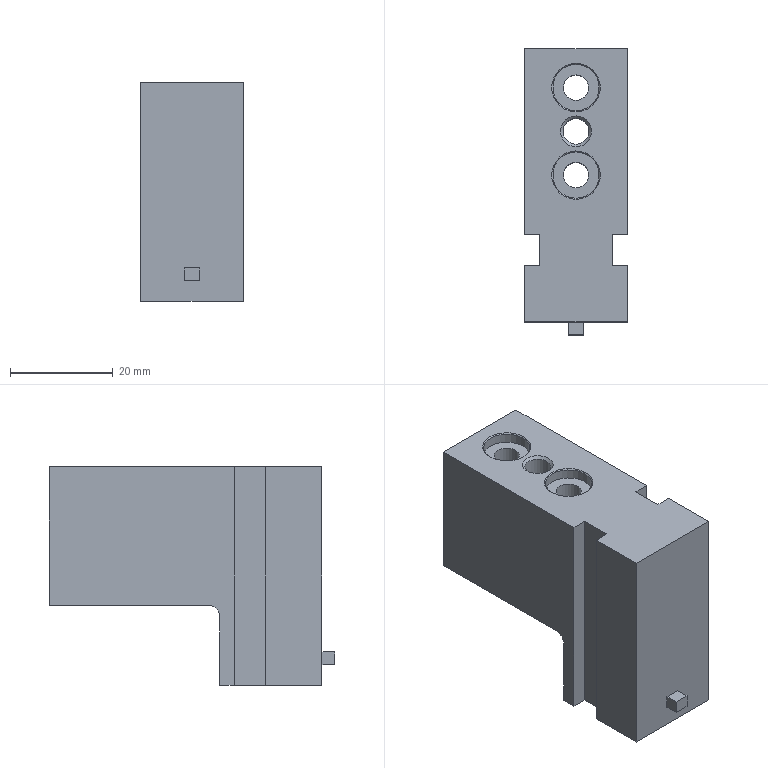Part | STEP file | 1254052_DHPS_35_A_2_14a---(GARRA) | 1 solid | 33 faces | box 20 x 55.5 x 42.5 mm | volume 31534 mm3 | plane 23 | cylinder 6 | cone 4 | commonest cylinder face diameters 4.917 x2 9 x2 4 x1 5 x1